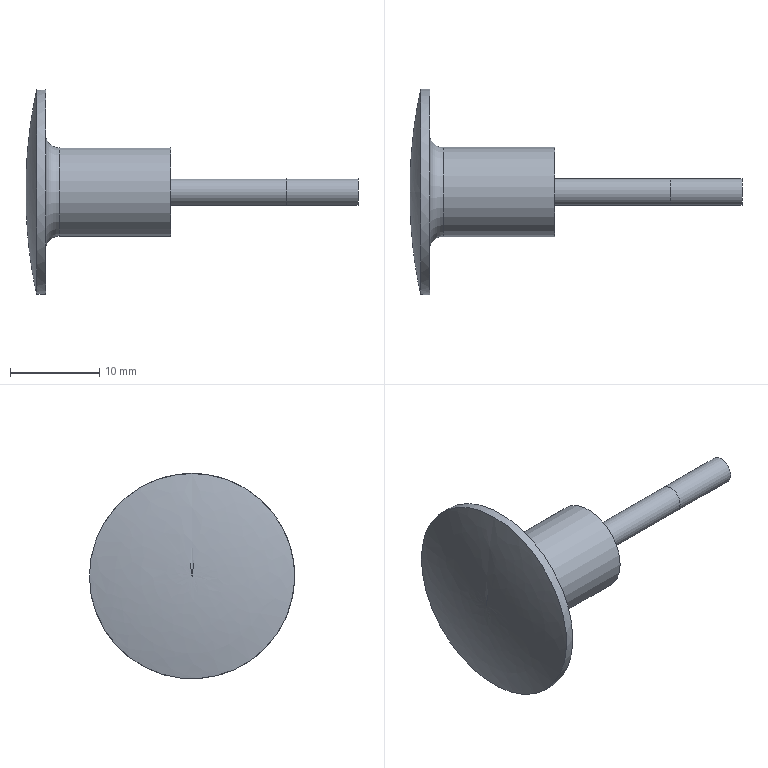Part | STEP file | 1-42.2 | 1 solid | 9 faces | box 37.201 x 23 x 23 mm | volume 1939 mm3 | cylinder 4 | plane 3 | spline 1 | torus 1 | commonest cylinder face diameters 3 x2 10 x1 23 x1
STEP:
#1=CARTESIAN_POINT('',(0.,0.,0.));
#2=DIRECTION('',(0.,0.,1.));
#3=DIRECTION('',(1.,0.,0.));
#4=AXIS2_PLACEMENT_3D('',#1,#2,#3);
#5=CARTESIAN_POINT('',(0.,11.5,0.));
#6=VERTEX_POINT('',#5);
#7=CARTESIAN_POINT('',(-1.,11.5,0.));
#8=VERTEX_POINT('',#7);
#9=CARTESIAN_POINT('',(0.,11.5,0.));
#10=DIRECTION('',(-1.,0.,0.));
#11=VECTOR('',#10,1.);
#12=LINE('',#9,#11);
#13=CARTESIAN_POINT('',(0.,0.,0.));
#14=DIRECTION('',(-1.,0.,0.));
#15=DIRECTION('',(0.,1.,0.));
#16=AXIS2_PLACEMENT_3D('',#13,#14,#15);
#17=CYLINDRICAL_SURFACE('',#16,11.5);
#18=CARTESIAN_POINT('',(6.283,0.));
#19=DIRECTION('',(0.,1.));
#20=VECTOR('',#19,1.);
#21=LINE('',#18,#20);
#22=(GEOMETRIC_REPRESENTATION_CONTEXT(2)PARAMETRIC_REPRESENTATION_CONTEXT()REPRESENTATION_CONTEXT('',''));
#23=DEFINITIONAL_REPRESENTATION('',(#21),#22);
#24=PCURVE('',#17,#23);
#25=CARTESIAN_POINT('',(0.,0.));
#26=DIRECTION('',(0.,1.));
#27=VECTOR('',#26,1.);
#28=LINE('',#25,#27);
#29=(GEOMETRIC_REPRESENTATION_CONTEXT(2)PARAMETRIC_REPRESENTATION_CONTEXT()REPRESENTATION_CONTEXT('',''));
#30=DEFINITIONAL_REPRESENTATION('',(#28),#29);
#31=PCURVE('',#17,#30);
#32=SEAM_CURVE('',#12,(#24,#31),.PCURVE_S1.);
#33=EDGE_CURVE('',#6,#8,#32,.T.);
#34=ORIENTED_EDGE('',*,*,#33,.T.);
#35=CARTESIAN_POINT('',(-1.,0.,11.5));
#36=VERTEX_POINT('',#35);
#37=CARTESIAN_POINT('',(-1.,0.,0.));
#38=DIRECTION('',(1.,0.,0.));
#39=DIRECTION('',(0.,1.,0.));
#40=AXIS2_PLACEMENT_3D('',#37,#38,#39);
#41=CIRCLE('',#40,11.5);
#42=CARTESIAN_POINT('',(6.283,1.));
#43=DIRECTION('',(-1.,0.));
#44=VECTOR('',#43,1.);
#45=LINE('',#42,#44);
#46=(GEOMETRIC_REPRESENTATION_CONTEXT(2)PARAMETRIC_REPRESENTATION_CONTEXT()REPRESENTATION_CONTEXT('',''));
#47=DEFINITIONAL_REPRESENTATION('',(#45),#46);
#48=PCURVE('',#17,#47);
#49=CARTESIAN_POINT('',(-1.,0.,11.5));
#50=CARTESIAN_POINT('',(-1.,-11.5,11.5));
#51=CARTESIAN_POINT('',(-1.,-11.5,0.));
#52=CARTESIAN_POINT('',(-1.,-11.5,-11.5));
#53=CARTESIAN_POINT('',(-1.,0.,-11.5));
#54=CARTESIAN_POINT('',(-1.,11.5,-11.5));
#55=CARTESIAN_POINT('',(-1.,11.5,0.));
#56=CARTESIAN_POINT('',(-1.,11.5,11.5));
#57=CARTESIAN_POINT('',(-1.,0.,11.5));
#58=CARTESIAN_POINT('',(-2.243,0.,5.817));
#59=CARTESIAN_POINT('',(-2.243,-5.817,5.817));
#60=CARTESIAN_POINT('',(-2.243,-5.817,0.));
#61=CARTESIAN_POINT('',(-2.243,-5.817,-5.817));
#62=CARTESIAN_POINT('',(-2.243,0.,-5.817));
#63=CARTESIAN_POINT('',(-2.243,5.817,-5.817));
#64=CARTESIAN_POINT('',(-2.243,5.817,0.));
#65=CARTESIAN_POINT('',(-2.243,5.817,5.817));
#66=CARTESIAN_POINT('',(-2.243,0.,5.817));
#67=CARTESIAN_POINT('',(-2.2,0.,0.));
#68=CARTESIAN_POINT('',(-2.2,0.,0.));
#69=CARTESIAN_POINT('',(-2.2,0.,0.));
#70=CARTESIAN_POINT('',(-2.2,0.,0.));
#71=CARTESIAN_POINT('',(-2.2,0.,0.));
#72=CARTESIAN_POINT('',(-2.2,0.,0.));
#73=CARTESIAN_POINT('',(-2.2,0.,0.));
#74=CARTESIAN_POINT('',(-2.2,0.,0.));
#75=CARTESIAN_POINT('',(-2.2,0.,0.));
#76=(BOUNDED_SURFACE()B_SPLINE_SURFACE(2,2,((#49,#50,#51,#52,#53,#54,#55,#56,#57),(#58,#59,#60,#61,#62,#63,#64,#65,#66),(#67,#68,#69,#70,#71,#72,#73,#74,#75)),.UNSPECIFIED.,.F.,.T.,.F.)B_SPLINE_SURFACE_WITH_KNOTS((3,3),(1,2,2,2,2,2,1),(0.,1.),(-0.25,0.,0.25,0.5,0.75,1.,1.25),.UNSPECIFIED.)GEOMETRIC_REPRESENTATION_ITEM()RATIONAL_B_SPLINE_SURFACE(((1.,0.7071,1.,0.7071,1.,0.7071,1.,0.7071,1.),(0.9938,0.7027,0.9938,0.7027,0.9938,0.7027,0.9938,0.7027,0.9938),(1.,0.7071,1.,0.7071,1.,0.7071,1.,0.7071,1.)))REPRESENTATION_ITEM('')SURFACE());
#77=CARTESIAN_POINT('',(0.,0.75));
#78=CARTESIAN_POINT('',(0.,0.7542));
#79=CARTESIAN_POINT('',(0.,0.7625));
#80=CARTESIAN_POINT('',(0.,0.7746));
#81=CARTESIAN_POINT('',(0.,0.7864));
#82=CARTESIAN_POINT('',(0.,0.798));
#83=CARTESIAN_POINT('',(0.,0.8094));
#84=CARTESIAN_POINT('',(0.,0.8206));
#85=CARTESIAN_POINT('',(0.,0.8316));
#86=CARTESIAN_POINT('',(0.,0.8426));
#87=CARTESIAN_POINT('',(0.,0.8534));
#88=CARTESIAN_POINT('',(0.,0.8642));
#89=CARTESIAN_POINT('',(0.,0.875));
#90=CARTESIAN_POINT('',(0.,0.8858));
#91=CARTESIAN_POINT('',(0.,0.8966));
#92=CARTESIAN_POINT('',(0.,0.9074));
#93=CARTESIAN_POINT('',(0.,0.9184));
#94=CARTESIAN_POINT('',(0.,0.9294));
#95=CARTESIAN_POINT('',(0.,0.9406));
#96=CARTESIAN_POINT('',(0.,0.952));
#97=CARTESIAN_POINT('',(0.,0.9636));
#98=CARTESIAN_POINT('',(0.,0.9754));
#99=CARTESIAN_POINT('',(0.,0.9875));
#100=CARTESIAN_POINT('',(0.,0.9958));
#101=CARTESIAN_POINT('',(0.,1.));
#102=B_SPLINE_CURVE_WITH_KNOTS('',3,(#77,#78,#79,#80,#81,#82,#83,#84,#85,#86,#87,#88,#89,#90,#91,#92,#93,#94,#95,#96,#97,#98,#99,#100,#101),.UNSPECIFIED.,.F.,.F.,(4,1,1,1,1,1,1,1,1,1,1,1,1,1,1,1,1,1,1,1,1,1,4),(0.,0.0714,0.1428,0.2142,0.2856,0.357,0.4284,0.4998,0.5712,0.6426,0.714,0.7854,0.8568,0.9282,0.9996,1.071,1.142,1.214,1.285,1.357,1.428,1.499,1.571),.QUASI_UNIFORM_KNOTS.);
#103=(GEOMETRIC_REPRESENTATION_CONTEXT(2)PARAMETRIC_REPRESENTATION_CONTEXT()REPRESENTATION_CONTEXT('',''));
#104=DEFINITIONAL_REPRESENTATION('',(#102),#103);
#105=PCURVE('',#76,#104);
#106=SURFACE_CURVE('',#41,(#48,#105),.PCURVE_S1.);
#107=EDGE_CURVE('',#8,#36,#106,.T.);
#108=ORIENTED_EDGE('',*,*,#107,.T.);
#109=CARTESIAN_POINT('',(-1.,0.,0.));
#110=DIRECTION('',(1.,0.,0.));
#111=DIRECTION('',(0.,0.,1.));
#112=AXIS2_PLACEMENT_3D('',#109,#110,#111);
#113=CIRCLE('',#112,11.5);
#114=CARTESIAN_POINT('',(4.712,1.));
#115=DIRECTION('',(-1.,0.));
#116=VECTOR('',#115,1.);
#117=LINE('',#114,#116);
#118=(GEOMETRIC_REPRESENTATION_CONTEXT(2)PARAMETRIC_REPRESENTATION_CONTEXT()REPRESENTATION_CONTEXT('',''));
#119=DEFINITIONAL_REPRESENTATION('',(#117),#118);
#120=PCURVE('',#17,#119);
#121=CARTESIAN_POINT('',(0.,0.));
#122=CARTESIAN_POINT('',(0.,0.0126));
#123=CARTESIAN_POINT('',(0.,0.03676));
#124=CARTESIAN_POINT('',(0.,0.07076));
#125=CARTESIAN_POINT('',(0.,0.1035));
#126=CARTESIAN_POINT('',(0.,0.1357));
#127=CARTESIAN_POINT('',(0.,0.1682));
#128=CARTESIAN_POINT('',(0.,0.2017));
#129=CARTESIAN_POINT('',(0.,0.2371));
#130=CARTESIAN_POINT('',(0.,0.2752));
#131=CARTESIAN_POINT('',(0.,0.3096));
#132=CARTESIAN_POINT('',(0.,0.3427));
#133=CARTESIAN_POINT('',(0.,0.375));
#134=CARTESIAN_POINT('',(0.,0.4073));
#135=CARTESIAN_POINT('',(0.,0.4404));
#136=CARTESIAN_POINT('',(0.,0.4748));
#137=CARTESIAN_POINT('',(0.,0.5129));
#138=CARTESIAN_POINT('',(0.,0.5483));
#139=CARTESIAN_POINT('',(0.,0.5818));
#140=CARTESIAN_POINT('',(0.,0.6143));
#141=CARTESIAN_POINT('',(0.,0.6465));
#142=CARTESIAN_POINT('',(0.,0.6792));
#143=CARTESIAN_POINT('',(0.,0.7132));
#144=CARTESIAN_POINT('',(0.,0.7374));
#145=CARTESIAN_POINT('',(0.,0.75));
#146=B_SPLINE_CURVE_WITH_KNOTS('',3,(#121,#122,#123,#124,#125,#126,#127,#128,#129,#130,#131,#132,#133,#134,#135,#136,#137,#138,#139,#140,#141,#142,#143,#144,#145),.UNSPECIFIED.,.F.,.F.,(4,1,1,1,1,1,1,1,1,1,1,1,1,1,1,1,1,1,1,1,1,1,4),(0.,0.2142,0.4284,0.6426,0.8568,1.071,1.285,1.499,1.714,1.928,2.142,2.356,2.57,2.785,2.999,3.213,3.427,3.641,3.856,4.07,4.284,4.498,4.712),.QUASI_UNIFORM_KNOTS.);
#147=(GEOMETRIC_REPRESENTATION_CONTEXT(2)PARAMETRIC_REPRESENTATION_CONTEXT()REPRESENTATION_CONTEXT('',''));
#148=DEFINITIONAL_REPRESENTATION('',(#146),#147);
#149=PCURVE('',#76,#148);
#150=SURFACE_CURVE('',#113,(#120,#149),.PCURVE_S1.);
#151=EDGE_CURVE('',#36,#8,#150,.T.);
#152=ORIENTED_EDGE('',*,*,#151,.T.);
#153=ORIENTED_EDGE('',*,*,#33,.F.);
#154=CARTESIAN_POINT('',(0.,0.,0.));
#155=DIRECTION('',(1.,0.,0.));
#156=DIRECTION('',(0.,1.,0.));
#157=AXIS2_PLACEMENT_3D('',#154,#155,#156);
#158=CIRCLE('',#157,11.5);
#159=CARTESIAN_POINT('',(6.283,0.));
#160=DIRECTION('',(-1.,0.));
#161=VECTOR('',#160,1.);
#162=LINE('',#159,#161);
#163=(GEOMETRIC_REPRESENTATION_CONTEXT(2)PARAMETRIC_REPRESENTATION_CONTEXT()REPRESENTATION_CONTEXT('',''));
#164=DEFINITIONAL_REPRESENTATION('',(#162),#163);
#165=PCURVE('',#17,#164);
#166=CARTESIAN_POINT('',(0.,-3.081,0.));
#167=DIRECTION('',(1.,0.,0.));
#168=DIRECTION('',(0.,0.,-1.));
#169=AXIS2_PLACEMENT_3D('',#166,#167,#168);
#170=PLANE('',#169);
#171=CARTESIAN_POINT('',(0.,3.081));
#172=DIRECTION('',(0.,1.));
#173=AXIS2_PLACEMENT_2D('',#171,#172);
#174=CIRCLE('',#173,11.5);
#175=(GEOMETRIC_REPRESENTATION_CONTEXT(2)PARAMETRIC_REPRESENTATION_CONTEXT()REPRESENTATION_CONTEXT('',''));
#176=DEFINITIONAL_REPRESENTATION('',(#174),#175);
#177=PCURVE('',#170,#176);
#178=SURFACE_CURVE('',#158,(#165,#177),.PCURVE_S1.);
#179=EDGE_CURVE('',#6,#6,#178,.T.);
#180=ORIENTED_EDGE('',*,*,#179,.F.);
#181=EDGE_LOOP('',(#34,#108,#152,#153,#180));
#182=FACE_BOUND('',#181,.T.);
#183=ADVANCED_FACE('',(#182),#17,.T.);
#184=CARTESIAN_POINT('',(-2.2,0.,0.));
#185=VERTEX_POINT('',#184);
#186=CARTESIAN_POINT('',(49.799,0.,0.3867));
#187=DIRECTION('',(0.,-1.,0.));
#188=DIRECTION('',(-0.9769,0.,0.2137));
#189=AXIS2_PLACEMENT_3D('',#186,#187,#188);
#190=CIRCLE('',#189,52.);
#191=CARTESIAN_POINT('',(0.,0.));
#192=CARTESIAN_POINT('',(0.01518,0.));
#193=CARTESIAN_POINT('',(0.04554,0.));
#194=CARTESIAN_POINT('',(0.09105,0.));
#195=CARTESIAN_POINT('',(0.1365,0.));
#196=CARTESIAN_POINT('',(0.182,0.));
#197=CARTESIAN_POINT('',(0.2275,0.));
#198=CARTESIAN_POINT('',(0.2729,0.));
#199=CARTESIAN_POINT('',(0.3183,0.));
#200=CARTESIAN_POINT('',(0.3638,0.));
#201=CARTESIAN_POINT('',(0.4092,0.));
#202=CARTESIAN_POINT('',(0.4546,0.));
#203=CARTESIAN_POINT('',(0.5,0.));
#204=CARTESIAN_POINT('',(0.5454,0.));
#205=CARTESIAN_POINT('',(0.5908,0.));
#206=CARTESIAN_POINT('',(0.6362,0.));
#207=CARTESIAN_POINT('',(0.6817,0.));
#208=CARTESIAN_POINT('',(0.7271,0.));
#209=CARTESIAN_POINT('',(0.7725,0.));
#210=CARTESIAN_POINT('',(0.818,0.));
#211=CARTESIAN_POINT('',(0.8635,0.));
#212=CARTESIAN_POINT('',(0.9089,0.));
#213=CARTESIAN_POINT('',(0.9545,0.));
#214=CARTESIAN_POINT('',(0.9848,0.));
#215=CARTESIAN_POINT('',(1.,0.));
#216=B_SPLINE_CURVE_WITH_KNOTS('',3,(#191,#192,#193,#194,#195,#196,#197,#198,#199,#200,#201,#202,#203,#204,#205,#206,#207,#208,#209,#210,#211,#212,#213,#214,#215),.UNSPECIFIED.,.F.,.F.,(4,1,1,1,1,1,1,1,1,1,1,1,1,1,1,1,1,1,1,1,1,1,4),(0.,0.01013,0.02026,0.03038,0.04051,0.05064,0.06077,0.0709,0.08102,0.09115,0.1013,0.1114,0.1215,0.1317,0.1418,0.1519,0.162,0.1722,0.1823,0.1924,0.2026,0.2127,0.2228),.QUASI_UNIFORM_KNOTS.);
#217=(GEOMETRIC_REPRESENTATION_CONTEXT(2)PARAMETRIC_REPRESENTATION_CONTEXT()REPRESENTATION_CONTEXT('',''));
#218=DEFINITIONAL_REPRESENTATION('',(#216),#217);
#219=PCURVE('',#76,#218);
#220=CARTESIAN_POINT('',(0.,1.));
#221=CARTESIAN_POINT('',(0.01518,1.));
#222=CARTESIAN_POINT('',(0.04554,1.));
#223=CARTESIAN_POINT('',(0.09105,1.));
#224=CARTESIAN_POINT('',(0.1365,1.));
#225=CARTESIAN_POINT('',(0.182,1.));
#226=CARTESIAN_POINT('',(0.2275,1.));
#227=CARTESIAN_POINT('',(0.2729,1.));
#228=CARTESIAN_POINT('',(0.3183,1.));
#229=CARTESIAN_POINT('',(0.3638,1.));
#230=CARTESIAN_POINT('',(0.4092,1.));
#231=CARTESIAN_POINT('',(0.4546,1.));
#232=CARTESIAN_POINT('',(0.5,1.));
#233=CARTESIAN_POINT('',(0.5454,1.));
#234=CARTESIAN_POINT('',(0.5908,1.));
#235=CARTESIAN_POINT('',(0.6362,1.));
#236=CARTESIAN_POINT('',(0.6817,1.));
#237=CARTESIAN_POINT('',(0.7271,1.));
#238=CARTESIAN_POINT('',(0.7725,1.));
#239=CARTESIAN_POINT('',(0.818,1.));
#240=CARTESIAN_POINT('',(0.8635,1.));
#241=CARTESIAN_POINT('',(0.9089,1.));
#242=CARTESIAN_POINT('',(0.9545,1.));
#243=CARTESIAN_POINT('',(0.9848,1.));
#244=CARTESIAN_POINT('',(1.,1.));
#245=B_SPLINE_CURVE_WITH_KNOTS('',3,(#220,#221,#222,#223,#224,#225,#226,#227,#228,#229,#230,#231,#232,#233,#234,#235,#236,#237,#238,#239,#240,#241,#242,#243,#244),.UNSPECIFIED.,.F.,.F.,(4,1,1,1,1,1,1,1,1,1,1,1,1,1,1,1,1,1,1,1,1,1,4),(0.,0.01013,0.02026,0.03038,0.04051,0.05064,0.06077,0.0709,0.08102,0.09115,0.1013,0.1114,0.1215,0.1317,0.1418,0.1519,0.162,0.1722,0.1823,0.1924,0.2026,0.2127,0.2228),.QUASI_UNIFORM_KNOTS.);
#246=(GEOMETRIC_REPRESENTATION_CONTEXT(2)PARAMETRIC_REPRESENTATION_CONTEXT()REPRESENTATION_CONTEXT('',''));
#247=DEFINITIONAL_REPRESENTATION('',(#245),#246);
#248=PCURVE('',#76,#247);
#249=SEAM_CURVE('',#190,(#219,#248),.PCURVE_S1.);
#250=EDGE_CURVE('',#36,#185,#249,.T.);
#251=ORIENTED_EDGE('',*,*,#250,.T.);
#252=ORIENTED_EDGE('',*,*,#250,.F.);
#253=ORIENTED_EDGE('',*,*,#107,.F.);
#254=ORIENTED_EDGE('',*,*,#151,.F.);
#255=EDGE_LOOP('',(#251,#252,#253,#254));
#256=FACE_BOUND('',#255,.T.);
#257=ADVANCED_FACE('',(#256),#76,.T.);
#258=CARTESIAN_POINT('',(14.,5.,0.));
#259=VERTEX_POINT('',#258);
#260=CARTESIAN_POINT('',(14.,0.,0.));
#261=DIRECTION('',(1.,0.,0.));
#262=DIRECTION('',(0.,1.,0.));
#263=AXIS2_PLACEMENT_3D('',#260,#261,#262);
#264=CIRCLE('',#263,5.);
#265=CARTESIAN_POINT('',(0.,0.,0.));
#266=DIRECTION('',(1.,0.,0.));
#267=DIRECTION('',(0.,1.,0.));
#268=AXIS2_PLACEMENT_3D('',#265,#266,#267);
#269=CYLINDRICAL_SURFACE('',#268,5.);
#270=CARTESIAN_POINT('',(0.,14.));
#271=DIRECTION('',(1.,0.));
#272=VECTOR('',#271,1.);
#273=LINE('',#270,#272);
#274=(GEOMETRIC_REPRESENTATION_CONTEXT(2)PARAMETRIC_REPRESENTATION_CONTEXT()REPRESENTATION_CONTEXT('',''));
#275=DEFINITIONAL_REPRESENTATION('',(#273),#274);
#276=PCURVE('',#269,#275);
#277=CARTESIAN_POINT('',(14.,-1.34,0.));
#278=DIRECTION('',(1.,0.,0.));
#279=DIRECTION('',(0.,0.,-1.));
#280=AXIS2_PLACEMENT_3D('',#277,#278,#279);
#281=PLANE('',#280);
#282=CARTESIAN_POINT('',(0.,1.34));
#283=DIRECTION('',(0.,1.));
#284=AXIS2_PLACEMENT_2D('',#282,#283);
#285=CIRCLE('',#284,5.);
#286=(GEOMETRIC_REPRESENTATION_CONTEXT(2)PARAMETRIC_REPRESENTATION_CONTEXT()REPRESENTATION_CONTEXT('',''));
#287=DEFINITIONAL_REPRESENTATION('',(#285),#286);
#288=PCURVE('',#281,#287);
#289=SURFACE_CURVE('',#264,(#276,#288),.PCURVE_S1.);
#290=EDGE_CURVE('',#259,#259,#289,.T.);
#291=ORIENTED_EDGE('',*,*,#290,.F.);
#292=CARTESIAN_POINT('',(1.5,5.,0.));
#293=VERTEX_POINT('',#292);
#294=CARTESIAN_POINT('',(1.5,5.,0.));
#295=DIRECTION('',(1.,0.,0.));
#296=VECTOR('',#295,1.);
#297=LINE('',#294,#296);
#298=CARTESIAN_POINT('',(0.,1.5));
#299=DIRECTION('',(0.,1.));
#300=VECTOR('',#299,1.);
#301=LINE('',#298,#300);
#302=(GEOMETRIC_REPRESENTATION_CONTEXT(2)PARAMETRIC_REPRESENTATION_CONTEXT()REPRESENTATION_CONTEXT('',''));
#303=DEFINITIONAL_REPRESENTATION('',(#301),#302);
#304=PCURVE('',#269,#303);
#305=CARTESIAN_POINT('',(6.283,1.5));
#306=DIRECTION('',(0.,1.));
#307=VECTOR('',#306,1.);
#308=LINE('',#305,#307);
#309=(GEOMETRIC_REPRESENTATION_CONTEXT(2)PARAMETRIC_REPRESENTATION_CONTEXT()REPRESENTATION_CONTEXT('',''));
#310=DEFINITIONAL_REPRESENTATION('',(#308),#309);
#311=PCURVE('',#269,#310);
#312=SEAM_CURVE('',#297,(#304,#311),.PCURVE_S1.);
#313=EDGE_CURVE('',#293,#259,#312,.T.);
#314=ORIENTED_EDGE('',*,*,#313,.F.);
#315=CARTESIAN_POINT('',(1.5,0.,0.));
#316=DIRECTION('',(-1.,0.,0.));
#317=DIRECTION('',(0.,1.,0.));
#318=AXIS2_PLACEMENT_3D('',#315,#316,#317);
#319=CIRCLE('',#318,5.);
#320=CARTESIAN_POINT('',(6.283,1.5));
#321=DIRECTION('',(-1.,0.));
#322=VECTOR('',#321,1.);
#323=LINE('',#320,#322);
#324=(GEOMETRIC_REPRESENTATION_CONTEXT(2)PARAMETRIC_REPRESENTATION_CONTEXT()REPRESENTATION_CONTEXT('',''));
#325=DEFINITIONAL_REPRESENTATION('',(#323),#324);
#326=PCURVE('',#269,#325);
#327=CARTESIAN_POINT('',(1.5,0.,0.));
#328=DIRECTION('',(1.,0.,0.));
#329=DIRECTION('',(0.,1.,0.));
#330=AXIS2_PLACEMENT_3D('',#327,#328,#329);
#331=TOROIDAL_SURFACE('',#330,6.5,1.5);
#332=CARTESIAN_POINT('',(6.283,3.142));
#333=DIRECTION('',(-1.,0.));
#334=VECTOR('',#333,1.);
#335=LINE('',#332,#334);
#336=(GEOMETRIC_REPRESENTATION_CONTEXT(2)PARAMETRIC_REPRESENTATION_CONTEXT()REPRESENTATION_CONTEXT('',''));
#337=DEFINITIONAL_REPRESENTATION('',(#335),#336);
#338=PCURVE('',#331,#337);
#339=SURFACE_CURVE('',#319,(#326,#338),.PCURVE_S1.);
#340=EDGE_CURVE('',#293,#293,#339,.T.);
#341=ORIENTED_EDGE('',*,*,#340,.F.);
#342=ORIENTED_EDGE('',*,*,#313,.T.);
#343=EDGE_LOOP('',(#291,#314,#341,#342));
#344=FACE_BOUND('',#343,.T.);
#345=ADVANCED_FACE('',(#344),#269,.T.);
#346=ORIENTED_EDGE('',*,*,#179,.T.);
#347=EDGE_LOOP('',(#346));
#348=FACE_BOUND('',#347,.T.);
#349=CARTESIAN_POINT('',(0.,6.5,0.));
#350=VERTEX_POINT('',#349);
#351=CARTESIAN_POINT('',(0.,0.,0.));
#352=DIRECTION('',(-1.,0.,0.));
#353=DIRECTION('',(0.,1.,0.));
#354=AXIS2_PLACEMENT_3D('',#351,#352,#353);
#355=CIRCLE('',#354,6.5);
#356=CARTESIAN_POINT('',(0.,9.581));
#357=CARTESIAN_POINT('',(11.258,9.581));
#358=CARTESIAN_POINT('',(5.629,-0.1686));
#359=CARTESIAN_POINT('',(0.,-9.919));
#360=CARTESIAN_POINT('',(-5.629,-0.1686));
#361=CARTESIAN_POINT('',(-11.258,9.581));
#362=CARTESIAN_POINT('',(0.,9.581));
#363=(BOUNDED_CURVE()B_SPLINE_CURVE(2,(#356,#357,#358,#359,#360,#361,#362),.UNSPECIFIED.,.T.,.F.)B_SPLINE_CURVE_WITH_KNOTS((1,2,2,2,2,1),(-2.094,0.,2.094,4.189,6.283,8.378),.UNSPECIFIED.)CURVE()GEOMETRIC_REPRESENTATION_ITEM()RATIONAL_B_SPLINE_CURVE((1.,0.5,1.,0.5,1.,0.5,1.))REPRESENTATION_ITEM(''));
#364=(GEOMETRIC_REPRESENTATION_CONTEXT(2)PARAMETRIC_REPRESENTATION_CONTEXT()REPRESENTATION_CONTEXT('',''));
#365=DEFINITIONAL_REPRESENTATION('',(#363),#364);
#366=PCURVE('',#170,#365);
#367=CARTESIAN_POINT('',(6.283,4.712));
#368=DIRECTION('',(-1.,0.));
#369=VECTOR('',#368,1.);
#370=LINE('',#367,#369);
#371=(GEOMETRIC_REPRESENTATION_CONTEXT(2)PARAMETRIC_REPRESENTATION_CONTEXT()REPRESENTATION_CONTEXT('',''));
#372=DEFINITIONAL_REPRESENTATION('',(#370),#371);
#373=PCURVE('',#331,#372);
#374=SURFACE_CURVE('',#355,(#366,#373),.PCURVE_S1.);
#375=EDGE_CURVE('',#350,#350,#374,.T.);
#376=ORIENTED_EDGE('',*,*,#375,.T.);
#377=EDGE_LOOP('',(#376));
#378=FACE_BOUND('',#377,.T.);
#379=ADVANCED_FACE('',(#348,#378),#170,.T.);
#380=CARTESIAN_POINT('',(1.5,6.5,0.));
#381=DIRECTION('',(0.,0.,-1.));
#382=DIRECTION('',(0.,-1.,0.));
#383=AXIS2_PLACEMENT_3D('',#380,#381,#382);
#384=CIRCLE('',#383,1.5);
#385=CARTESIAN_POINT('',(0.,3.142));
#386=DIRECTION('',(0.,1.));
#387=VECTOR('',#386,1.);
#388=LINE('',#385,#387);
#389=(GEOMETRIC_REPRESENTATION_CONTEXT(2)PARAMETRIC_REPRESENTATION_CONTEXT()REPRESENTATION_CONTEXT('',''));
#390=DEFINITIONAL_REPRESENTATION('',(#388),#389);
#391=PCURVE('',#331,#390);
#392=CARTESIAN_POINT('',(6.283,3.142));
#393=DIRECTION('',(0.,1.));
#394=VECTOR('',#393,1.);
#395=LINE('',#392,#394);
#396=(GEOMETRIC_REPRESENTATION_CONTEXT(2)PARAMETRIC_REPRESENTATION_CONTEXT()REPRESENTATION_CONTEXT('',''));
#397=DEFINITIONAL_REPRESENTATION('',(#395),#396);
#398=PCURVE('',#331,#397);
#399=SEAM_CURVE('',#384,(#391,#398),.PCURVE_S1.);
#400=EDGE_CURVE('',#293,#350,#399,.T.);
#401=ORIENTED_EDGE('',*,*,#400,.F.);
#402=ORIENTED_EDGE('',*,*,#340,.F.);
#403=ORIENTED_EDGE('',*,*,#400,.T.);
#404=ORIENTED_EDGE('',*,*,#375,.T.);
#405=EDGE_LOOP('',(#401,#402,#403,#404));
#406=FACE_BOUND('',#405,.F.);
#407=ADVANCED_FACE('',(#406),#331,.F.);
#408=ORIENTED_EDGE('',*,*,#290,.T.);
#409=EDGE_LOOP('',(#408));
#410=FACE_BOUND('',#409,.T.);
#411=CARTESIAN_POINT('',(14.,1.5,0.));
#412=VERTEX_POINT('',#411);
#413=CARTESIAN_POINT('',(14.,0.,0.));
#414=DIRECTION('',(1.,0.,0.));
#415=DIRECTION('',(0.,1.,0.));
#416=AXIS2_PLACEMENT_3D('',#413,#414,#415);
#417=CIRCLE('',#416,1.5);
#418=CARTESIAN_POINT('',(0.,1.34));
#419=DIRECTION('',(0.,1.));
#420=AXIS2_PLACEMENT_2D('',#418,#419);
#421=CIRCLE('',#420,1.5);
#422=(GEOMETRIC_REPRESENTATION_CONTEXT(2)PARAMETRIC_REPRESENTATION_CONTEXT()REPRESENTATION_CONTEXT('',''));
#423=DEFINITIONAL_REPRESENTATION('',(#421),#422);
#424=PCURVE('',#281,#423);
#425=CARTESIAN_POINT('',(14.,0.,0.));
#426=DIRECTION('',(1.,0.,0.));
#427=DIRECTION('',(0.,1.,0.));
#428=AXIS2_PLACEMENT_3D('',#425,#426,#427);
#429=CYLINDRICAL_SURFACE('',#428,1.5);
#430=CARTESIAN_POINT('',(0.,0.));
#431=DIRECTION('',(1.,0.));
#432=VECTOR('',#431,1.);
#433=LINE('',#430,#432);
#434=(GEOMETRIC_REPRESENTATION_CONTEXT(2)PARAMETRIC_REPRESENTATION_CONTEXT()REPRESENTATION_CONTEXT('',''));
#435=DEFINITIONAL_REPRESENTATION('',(#433),#434);
#436=PCURVE('',#429,#435);
#437=SURFACE_CURVE('',#417,(#424,#436),.PCURVE_S1.);
#438=EDGE_CURVE('',#412,#412,#437,.T.);
#439=ORIENTED_EDGE('',*,*,#438,.F.);
#440=EDGE_LOOP('',(#439));
#441=FACE_BOUND('',#440,.T.);
#442=ADVANCED_FACE('',(#410,#441),#281,.T.);
#443=CARTESIAN_POINT('',(35.,1.5,0.));
#444=VERTEX_POINT('',#443);
#445=CARTESIAN_POINT('',(35.,0.,0.));
#446=DIRECTION('',(1.,0.,0.));
#447=DIRECTION('',(0.,1.,0.));
#448=AXIS2_PLACEMENT_3D('',#445,#446,#447);
#449=CIRCLE('',#448,1.5);
#450=CARTESIAN_POINT('',(35.,-0.4019,0.));
#451=DIRECTION('',(1.,0.,0.));
#452=DIRECTION('',(0.,1.,0.));
#453=AXIS2_PLACEMENT_3D('',#450,#451,#452);
#454=PLANE('',#453);
#455=CARTESIAN_POINT('',(0.4019,0.));
#456=DIRECTION('',(1.,0.));
#457=AXIS2_PLACEMENT_2D('',#455,#456);
#458=CIRCLE('',#457,1.5);
#459=(GEOMETRIC_REPRESENTATION_CONTEXT(2)PARAMETRIC_REPRESENTATION_CONTEXT()REPRESENTATION_CONTEXT('',''));
#460=DEFINITIONAL_REPRESENTATION('',(#458),#459);
#461=PCURVE('',#454,#460);
#462=CARTESIAN_POINT('',(27.,0.,0.));
#463=DIRECTION('',(1.,0.,0.));
#464=DIRECTION('',(0.,1.,0.));
#465=AXIS2_PLACEMENT_3D('',#462,#463,#464);
#466=CYLINDRICAL_SURFACE('',#465,1.5);
#467=CARTESIAN_POINT('',(0.,8.));
#468=DIRECTION('',(1.,0.));
#469=VECTOR('',#468,1.);
#470=LINE('',#467,#469);
#471=(GEOMETRIC_REPRESENTATION_CONTEXT(2)PARAMETRIC_REPRESENTATION_CONTEXT()REPRESENTATION_CONTEXT('',''));
#472=DEFINITIONAL_REPRESENTATION('',(#470),#471);
#473=PCURVE('',#466,#472);
#474=SURFACE_CURVE('',#449,(#461,#473),.PCURVE_S1.);
#475=EDGE_CURVE('',#444,#444,#474,.T.);
#476=ORIENTED_EDGE('',*,*,#475,.T.);
#477=EDGE_LOOP('',(#476));
#478=FACE_BOUND('',#477,.T.);
#479=ADVANCED_FACE('',(#478),#454,.T.);
#480=ORIENTED_EDGE('',*,*,#438,.T.);
#481=CARTESIAN_POINT('',(27.,1.5,0.));
#482=VERTEX_POINT('',#481);
#483=CARTESIAN_POINT('',(14.,1.5,0.));
#484=DIRECTION('',(1.,0.,0.));
#485=VECTOR('',#484,1.);
#486=LINE('',#483,#485);
#487=CARTESIAN_POINT('',(6.283,0.));
#488=DIRECTION('',(0.,1.));
#489=VECTOR('',#488,1.);
#490=LINE('',#487,#489);
#491=(GEOMETRIC_REPRESENTATION_CONTEXT(2)PARAMETRIC_REPRESENTATION_CONTEXT()REPRESENTATION_CONTEXT('',''));
#492=DEFINITIONAL_REPRESENTATION('',(#490),#491);
#493=PCURVE('',#429,#492);
#494=CARTESIAN_POINT('',(0.,0.));
#495=DIRECTION('',(0.,1.));
#496=VECTOR('',#495,1.);
#497=LINE('',#494,#496);
#498=(GEOMETRIC_REPRESENTATION_CONTEXT(2)PARAMETRIC_REPRESENTATION_CONTEXT()REPRESENTATION_CONTEXT('',''));
#499=DEFINITIONAL_REPRESENTATION('',(#497),#498);
#500=PCURVE('',#429,#499);
#501=SEAM_CURVE('',#486,(#493,#500),.PCURVE_S1.);
#502=EDGE_CURVE('',#412,#482,#501,.T.);
#503=ORIENTED_EDGE('',*,*,#502,.T.);
#504=CARTESIAN_POINT('',(27.,0.,0.));
#505=DIRECTION('',(1.,0.,0.));
#506=DIRECTION('',(0.,1.,0.));
#507=AXIS2_PLACEMENT_3D('',#504,#505,#506);
#508=CIRCLE('',#507,1.5);
#509=CARTESIAN_POINT('',(0.,13.));
#510=DIRECTION('',(1.,0.));
#511=VECTOR('',#510,1.);
#512=LINE('',#509,#511);
#513=(GEOMETRIC_REPRESENTATION_CONTEXT(2)PARAMETRIC_REPRESENTATION_CONTEXT()REPRESENTATION_CONTEXT('',''));
#514=DEFINITIONAL_REPRESENTATION('',(#512),#513);
#515=PCURVE('',#429,#514);
#516=CARTESIAN_POINT('',(0.,0.));
#517=DIRECTION('',(1.,0.));
#518=VECTOR('',#517,1.);
#519=LINE('',#516,#518);
#520=(GEOMETRIC_REPRESENTATION_CONTEXT(2)PARAMETRIC_REPRESENTATION_CONTEXT()REPRESENTATION_CONTEXT('',''));
#521=DEFINITIONAL_REPRESENTATION('',(#519),#520);
#522=PCURVE('',#466,#521);
#523=SURFACE_CURVE('',#508,(#515,#522),.PCURVE_S1.);
#524=EDGE_CURVE('',#482,#482,#523,.T.);
#525=ORIENTED_EDGE('',*,*,#524,.F.);
#526=ORIENTED_EDGE('',*,*,#502,.F.);
#527=EDGE_LOOP('',(#480,#503,#525,#526));
#528=FACE_BOUND('',#527,.T.);
#529=ADVANCED_FACE('',(#528),#429,.T.);
#530=ORIENTED_EDGE('',*,*,#475,.F.);
#531=CARTESIAN_POINT('',(27.,1.5,0.));
#532=DIRECTION('',(1.,0.,0.));
#533=VECTOR('',#532,1.);
#534=LINE('',#531,#533);
#535=CARTESIAN_POINT('',(0.,0.));
#536=DIRECTION('',(0.,1.));
#537=VECTOR('',#536,1.);
#538=LINE('',#535,#537);
#539=(GEOMETRIC_REPRESENTATION_CONTEXT(2)PARAMETRIC_REPRESENTATION_CONTEXT()REPRESENTATION_CONTEXT('',''));
#540=DEFINITIONAL_REPRESENTATION('',(#538),#539);
#541=PCURVE('',#466,#540);
#542=CARTESIAN_POINT('',(6.283,0.));
#543=DIRECTION('',(0.,1.));
#544=VECTOR('',#543,1.);
#545=LINE('',#542,#544);
#546=(GEOMETRIC_REPRESENTATION_CONTEXT(2)PARAMETRIC_REPRESENTATION_CONTEXT()REPRESENTATION_CONTEXT('',''));
#547=DEFINITIONAL_REPRESENTATION('',(#545),#546);
#548=PCURVE('',#466,#547);
#549=SEAM_CURVE('',#534,(#541,#548),.PCURVE_S1.);
#550=EDGE_CURVE('',#482,#444,#549,.T.);
#551=ORIENTED_EDGE('',*,*,#550,.F.);
#552=ORIENTED_EDGE('',*,*,#524,.T.);
#553=ORIENTED_EDGE('',*,*,#550,.T.);
#554=EDGE_LOOP('',(#530,#551,#552,#553));
#555=FACE_BOUND('',#554,.T.);
#556=ADVANCED_FACE('',(#555),#466,.T.);
#557=CLOSED_SHELL('',(#183,#257,#345,#379,#407,#442,#479,#529,#556));
#558=MANIFOLD_SOLID_BREP('',#557);
#559=(LENGTH_UNIT()NAMED_UNIT(*)SI_UNIT(.MILLI.,.METRE.));
#560=UNCERTAINTY_MEASURE_WITH_UNIT(LENGTH_MEASURE(0.0000001),#559,'','');
#561=(NAMED_UNIT(*)PLANE_ANGLE_UNIT()SI_UNIT($,.RADIAN.));
#562=(NAMED_UNIT(*)SI_UNIT($,.STERADIAN.)SOLID_ANGLE_UNIT());
#563=(GEOMETRIC_REPRESENTATION_CONTEXT(3)GLOBAL_UNCERTAINTY_ASSIGNED_CONTEXT((#560))GLOBAL_UNIT_ASSIGNED_CONTEXT((#559,#561,#562))REPRESENTATION_CONTEXT('',''));
#564=ADVANCED_BREP_SHAPE_REPRESENTATION('',(#4,#558),#563);